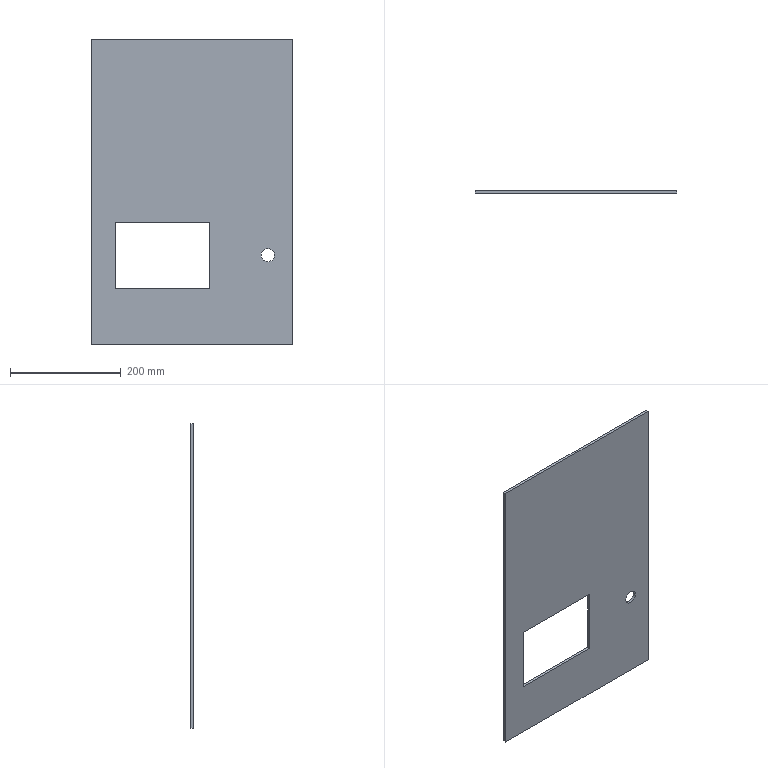Part | NX | 1 solid | 12 faces | box 365 x 5 x 550 mm | volume 899488 mm3 | plane 10 | cylinder 2 | commonest cylinder face diameters 24 x2
STEP:
#1=CARTESIAN_POINT('',(189.68,5.,13.));
#2=VERTEX_POINT('',#1);
#3=CARTESIAN_POINT('',(189.68,5.,-11.));
#4=VERTEX_POINT('',#3);
#5=CARTESIAN_POINT('',(189.68,5.,1.));
#6=DIRECTION('',(0.,-1.,0.));
#7=DIRECTION('',(0.,0.,-1.));
#8=AXIS2_PLACEMENT_3D('',#5,#6,#7);
#9=CIRCLE('',#8,12.);
#10=EDGE_CURVE('',#2,#4,#9,.T.);
#11=ORIENTED_EDGE('',*,*,#10,.F.);
#12=CARTESIAN_POINT('',(189.68,0.,13.));
#13=VERTEX_POINT('',#12);
#14=CARTESIAN_POINT('',(189.68,5.,13.));
#15=DIRECTION('',(0.,1.,0.));
#16=VECTOR('',#15,1.);
#17=LINE('',#14,#16);
#18=EDGE_CURVE('',#13,#2,#17,.T.);
#19=ORIENTED_EDGE('',*,*,#18,.F.);
#20=CARTESIAN_POINT('',(189.68,0.,-11.));
#21=VERTEX_POINT('',#20);
#22=CARTESIAN_POINT('',(189.68,0.,1.));
#23=DIRECTION('',(0.,-1.,0.));
#24=DIRECTION('',(0.,0.,-1.));
#25=AXIS2_PLACEMENT_3D('',#22,#23,#24);
#26=CIRCLE('',#25,12.);
#27=EDGE_CURVE('',#13,#21,#26,.T.);
#28=ORIENTED_EDGE('',*,*,#27,.T.);
#29=CARTESIAN_POINT('',(189.68,5.,-11.));
#30=DIRECTION('',(0.,1.,0.));
#31=VECTOR('',#30,1.);
#32=LINE('',#29,#31);
#33=EDGE_CURVE('',#21,#4,#32,.T.);
#34=ORIENTED_EDGE('',*,*,#33,.T.);
#35=EDGE_LOOP('',(#11,#19,#28,#34));
#36=FACE_OUTER_BOUND('',#35,.T.);
#37=CARTESIAN_POINT('',(189.68,5.,1.));
#38=DIRECTION('',(0.,-1.,0.));
#39=DIRECTION('',(0.,0.,-1.));
#40=AXIS2_PLACEMENT_3D('',#37,#38,#39);
#41=CYLINDRICAL_SURFACE('',#40,12.);
#42=ADVANCED_FACE('',(#36),#41,.F.);
#43=CARTESIAN_POINT('',(189.68,5.,1.));
#44=DIRECTION('',(0.,-1.,0.));
#45=DIRECTION('',(0.,0.,-1.));
#46=AXIS2_PLACEMENT_3D('',#43,#44,#45);
#47=CIRCLE('',#46,12.);
#48=EDGE_CURVE('',#4,#2,#47,.T.);
#49=ORIENTED_EDGE('',*,*,#48,.T.);
#50=ORIENTED_EDGE('',*,*,#10,.T.);
#51=EDGE_LOOP('',(#49,#50));
#52=FACE_BOUND('',#51,.T.);
#53=CARTESIAN_POINT('',(235.,5.,-160.));
#54=VERTEX_POINT('',#53);
#55=CARTESIAN_POINT('',(-130.,5.,-160.));
#56=VERTEX_POINT('',#55);
#57=CARTESIAN_POINT('',(-165.,5.,-160.));
#58=DIRECTION('',(-1.,0.,0.));
#59=VECTOR('',#58,1.);
#60=LINE('',#57,#59);
#61=EDGE_CURVE('',#54,#56,#60,.T.);
#62=ORIENTED_EDGE('',*,*,#61,.T.);
#63=CARTESIAN_POINT('',(-130.,5.,390.));
#64=VERTEX_POINT('',#63);
#65=CARTESIAN_POINT('',(-130.,5.,-160.));
#66=DIRECTION('',(0.,0.,-1.));
#67=VECTOR('',#66,1.);
#68=LINE('',#65,#67);
#69=EDGE_CURVE('',#64,#56,#68,.T.);
#70=ORIENTED_EDGE('',*,*,#69,.F.);
#71=CARTESIAN_POINT('',(235.,5.,390.));
#72=VERTEX_POINT('',#71);
#73=CARTESIAN_POINT('',(-165.,5.,390.));
#74=DIRECTION('',(1.,0.,0.));
#75=VECTOR('',#74,1.);
#76=LINE('',#73,#75);
#77=EDGE_CURVE('',#64,#72,#76,.T.);
#78=ORIENTED_EDGE('',*,*,#77,.T.);
#79=CARTESIAN_POINT('',(235.,5.,-160.));
#80=DIRECTION('',(0.,0.,-1.));
#81=VECTOR('',#80,1.);
#82=LINE('',#79,#81);
#83=EDGE_CURVE('',#72,#54,#82,.T.);
#84=ORIENTED_EDGE('',*,*,#83,.T.);
#85=EDGE_LOOP('',(#62,#70,#78,#84));
#86=FACE_BOUND('',#85,.T.);
#87=CARTESIAN_POINT('',(85.,5.,60.));
#88=VERTEX_POINT('',#87);
#89=CARTESIAN_POINT('',(85.,5.,-60.));
#90=VERTEX_POINT('',#89);
#91=CARTESIAN_POINT('',(85.,5.,-60.));
#92=DIRECTION('',(0.,0.,-1.));
#93=VECTOR('',#92,1.);
#94=LINE('',#91,#93);
#95=EDGE_CURVE('',#88,#90,#94,.T.);
#96=ORIENTED_EDGE('',*,*,#95,.F.);
#97=CARTESIAN_POINT('',(-85.,5.,60.));
#98=VERTEX_POINT('',#97);
#99=CARTESIAN_POINT('',(-85.,5.,60.));
#100=DIRECTION('',(1.,0.,0.));
#101=VECTOR('',#100,1.);
#102=LINE('',#99,#101);
#103=EDGE_CURVE('',#98,#88,#102,.T.);
#104=ORIENTED_EDGE('',*,*,#103,.F.);
#105=CARTESIAN_POINT('',(-85.,5.,-60.));
#106=VERTEX_POINT('',#105);
#107=CARTESIAN_POINT('',(-85.,5.,-60.));
#108=DIRECTION('',(0.,0.,1.));
#109=VECTOR('',#108,1.);
#110=LINE('',#107,#109);
#111=EDGE_CURVE('',#106,#98,#110,.T.);
#112=ORIENTED_EDGE('',*,*,#111,.F.);
#113=CARTESIAN_POINT('',(-85.,5.,-60.));
#114=DIRECTION('',(-1.,0.,0.));
#115=VECTOR('',#114,1.);
#116=LINE('',#113,#115);
#117=EDGE_CURVE('',#90,#106,#116,.T.);
#118=ORIENTED_EDGE('',*,*,#117,.F.);
#119=EDGE_LOOP('',(#96,#104,#112,#118));
#120=FACE_BOUND('',#119,.T.);
#121=CARTESIAN_POINT('',(235.,5.,-160.));
#122=DIRECTION('',(0.,-1.,0.));
#123=DIRECTION('',(0.,0.,-1.));
#124=AXIS2_PLACEMENT_3D('',#121,#122,#123);
#125=PLANE('',#124);
#126=ADVANCED_FACE('',(#52,#86,#120),#125,.F.);
#127=CARTESIAN_POINT('',(189.68,0.,1.));
#128=DIRECTION('',(0.,-1.,0.));
#129=DIRECTION('',(0.,0.,-1.));
#130=AXIS2_PLACEMENT_3D('',#127,#128,#129);
#131=CIRCLE('',#130,12.);
#132=EDGE_CURVE('',#21,#13,#131,.T.);
#133=ORIENTED_EDGE('',*,*,#132,.F.);
#134=ORIENTED_EDGE('',*,*,#27,.F.);
#135=EDGE_LOOP('',(#133,#134));
#136=FACE_BOUND('',#135,.T.);
#137=CARTESIAN_POINT('',(-130.,0.,-160.));
#138=VERTEX_POINT('',#137);
#139=CARTESIAN_POINT('',(-130.,0.,390.));
#140=VERTEX_POINT('',#139);
#141=CARTESIAN_POINT('',(-130.,0.,-160.));
#142=DIRECTION('',(0.,0.,1.));
#143=VECTOR('',#142,1.);
#144=LINE('',#141,#143);
#145=EDGE_CURVE('',#138,#140,#144,.T.);
#146=ORIENTED_EDGE('',*,*,#145,.F.);
#147=CARTESIAN_POINT('',(235.,0.,-160.));
#148=VERTEX_POINT('',#147);
#149=CARTESIAN_POINT('',(-165.,0.,-160.));
#150=DIRECTION('',(-1.,0.,0.));
#151=VECTOR('',#150,1.);
#152=LINE('',#149,#151);
#153=EDGE_CURVE('',#148,#138,#152,.T.);
#154=ORIENTED_EDGE('',*,*,#153,.F.);
#155=CARTESIAN_POINT('',(235.,0.,390.));
#156=VERTEX_POINT('',#155);
#157=CARTESIAN_POINT('',(235.,0.,-160.));
#158=DIRECTION('',(0.,0.,-1.));
#159=VECTOR('',#158,1.);
#160=LINE('',#157,#159);
#161=EDGE_CURVE('',#156,#148,#160,.T.);
#162=ORIENTED_EDGE('',*,*,#161,.F.);
#163=CARTESIAN_POINT('',(-165.,0.,390.));
#164=DIRECTION('',(1.,0.,0.));
#165=VECTOR('',#164,1.);
#166=LINE('',#163,#165);
#167=EDGE_CURVE('',#140,#156,#166,.T.);
#168=ORIENTED_EDGE('',*,*,#167,.F.);
#169=EDGE_LOOP('',(#146,#154,#162,#168));
#170=FACE_BOUND('',#169,.T.);
#171=CARTESIAN_POINT('',(-85.,0.,60.));
#172=VERTEX_POINT('',#171);
#173=CARTESIAN_POINT('',(85.,0.,60.));
#174=VERTEX_POINT('',#173);
#175=CARTESIAN_POINT('',(-85.,0.,60.));
#176=DIRECTION('',(1.,0.,0.));
#177=VECTOR('',#176,1.);
#178=LINE('',#175,#177);
#179=EDGE_CURVE('',#172,#174,#178,.T.);
#180=ORIENTED_EDGE('',*,*,#179,.T.);
#181=CARTESIAN_POINT('',(85.,0.,-60.));
#182=VERTEX_POINT('',#181);
#183=CARTESIAN_POINT('',(85.,0.,-60.));
#184=DIRECTION('',(0.,0.,-1.));
#185=VECTOR('',#184,1.);
#186=LINE('',#183,#185);
#187=EDGE_CURVE('',#174,#182,#186,.T.);
#188=ORIENTED_EDGE('',*,*,#187,.T.);
#189=CARTESIAN_POINT('',(-85.,0.,-60.));
#190=VERTEX_POINT('',#189);
#191=CARTESIAN_POINT('',(-85.,0.,-60.));
#192=DIRECTION('',(-1.,0.,0.));
#193=VECTOR('',#192,1.);
#194=LINE('',#191,#193);
#195=EDGE_CURVE('',#182,#190,#194,.T.);
#196=ORIENTED_EDGE('',*,*,#195,.T.);
#197=CARTESIAN_POINT('',(-85.,0.,-60.));
#198=DIRECTION('',(0.,0.,1.));
#199=VECTOR('',#198,1.);
#200=LINE('',#197,#199);
#201=EDGE_CURVE('',#190,#172,#200,.T.);
#202=ORIENTED_EDGE('',*,*,#201,.T.);
#203=EDGE_LOOP('',(#180,#188,#196,#202));
#204=FACE_BOUND('',#203,.T.);
#205=CARTESIAN_POINT('',(235.,0.,-160.));
#206=DIRECTION('',(0.,-1.,0.));
#207=DIRECTION('',(0.,0.,-1.));
#208=AXIS2_PLACEMENT_3D('',#205,#206,#207);
#209=PLANE('',#208);
#210=ADVANCED_FACE('',(#136,#170,#204),#209,.T.);
#211=ORIENTED_EDGE('',*,*,#153,.T.);
#212=CARTESIAN_POINT('',(-130.,-5.,-160.));
#213=DIRECTION('',(0.,1.,0.));
#214=VECTOR('',#213,1.);
#215=LINE('',#212,#214);
#216=EDGE_CURVE('',#138,#56,#215,.T.);
#217=ORIENTED_EDGE('',*,*,#216,.T.);
#218=ORIENTED_EDGE('',*,*,#61,.F.);
#219=CARTESIAN_POINT('',(235.,5.,-160.));
#220=DIRECTION('',(0.,-1.,0.));
#221=VECTOR('',#220,1.);
#222=LINE('',#219,#221);
#223=EDGE_CURVE('',#54,#148,#222,.T.);
#224=ORIENTED_EDGE('',*,*,#223,.T.);
#225=EDGE_LOOP('',(#211,#217,#218,#224));
#226=FACE_OUTER_BOUND('',#225,.T.);
#227=CARTESIAN_POINT('',(-165.,5.,-160.));
#228=DIRECTION('',(0.,0.,1.));
#229=DIRECTION('',(1.,0.,0.));
#230=AXIS2_PLACEMENT_3D('',#227,#228,#229);
#231=PLANE('',#230);
#232=ADVANCED_FACE('',(#226),#231,.F.);
#233=ORIENTED_EDGE('',*,*,#77,.F.);
#234=CARTESIAN_POINT('',(-130.,5.,390.));
#235=DIRECTION('',(0.,-1.,0.));
#236=VECTOR('',#235,1.);
#237=LINE('',#234,#236);
#238=EDGE_CURVE('',#64,#140,#237,.T.);
#239=ORIENTED_EDGE('',*,*,#238,.T.);
#240=ORIENTED_EDGE('',*,*,#167,.T.);
#241=CARTESIAN_POINT('',(235.,5.,390.));
#242=DIRECTION('',(0.,-1.,0.));
#243=VECTOR('',#242,1.);
#244=LINE('',#241,#243);
#245=EDGE_CURVE('',#72,#156,#244,.T.);
#246=ORIENTED_EDGE('',*,*,#245,.F.);
#247=EDGE_LOOP('',(#233,#239,#240,#246));
#248=FACE_OUTER_BOUND('',#247,.T.);
#249=CARTESIAN_POINT('',(-165.,5.,390.));
#250=DIRECTION('',(0.,0.,-1.));
#251=DIRECTION('',(-1.,0.,0.));
#252=AXIS2_PLACEMENT_3D('',#249,#250,#251);
#253=PLANE('',#252);
#254=ADVANCED_FACE('',(#248),#253,.F.);
#255=ORIENTED_EDGE('',*,*,#161,.T.);
#256=ORIENTED_EDGE('',*,*,#223,.F.);
#257=ORIENTED_EDGE('',*,*,#83,.F.);
#258=ORIENTED_EDGE('',*,*,#245,.T.);
#259=EDGE_LOOP('',(#255,#256,#257,#258));
#260=FACE_OUTER_BOUND('',#259,.T.);
#261=CARTESIAN_POINT('',(235.,5.,-160.));
#262=DIRECTION('',(-1.,0.,0.));
#263=DIRECTION('',(0.,0.,1.));
#264=AXIS2_PLACEMENT_3D('',#261,#262,#263);
#265=PLANE('',#264);
#266=ADVANCED_FACE('',(#260),#265,.F.);
#267=ORIENTED_EDGE('',*,*,#187,.F.);
#268=CARTESIAN_POINT('',(85.,5.,60.));
#269=DIRECTION('',(0.,-1.,0.));
#270=VECTOR('',#269,1.);
#271=LINE('',#268,#270);
#272=EDGE_CURVE('',#88,#174,#271,.T.);
#273=ORIENTED_EDGE('',*,*,#272,.F.);
#274=ORIENTED_EDGE('',*,*,#95,.T.);
#275=CARTESIAN_POINT('',(85.,5.,-60.));
#276=DIRECTION('',(0.,-1.,0.));
#277=VECTOR('',#276,1.);
#278=LINE('',#275,#277);
#279=EDGE_CURVE('',#90,#182,#278,.T.);
#280=ORIENTED_EDGE('',*,*,#279,.T.);
#281=EDGE_LOOP('',(#267,#273,#274,#280));
#282=FACE_OUTER_BOUND('',#281,.T.);
#283=CARTESIAN_POINT('',(85.,5.,-60.));
#284=DIRECTION('',(-1.,0.,0.));
#285=DIRECTION('',(0.,0.,1.));
#286=AXIS2_PLACEMENT_3D('',#283,#284,#285);
#287=PLANE('',#286);
#288=ADVANCED_FACE('',(#282),#287,.T.);
#289=ORIENTED_EDGE('',*,*,#195,.F.);
#290=ORIENTED_EDGE('',*,*,#279,.F.);
#291=ORIENTED_EDGE('',*,*,#117,.T.);
#292=CARTESIAN_POINT('',(-85.,5.,-60.));
#293=DIRECTION('',(0.,-1.,0.));
#294=VECTOR('',#293,1.);
#295=LINE('',#292,#294);
#296=EDGE_CURVE('',#106,#190,#295,.T.);
#297=ORIENTED_EDGE('',*,*,#296,.T.);
#298=EDGE_LOOP('',(#289,#290,#291,#297));
#299=FACE_OUTER_BOUND('',#298,.T.);
#300=CARTESIAN_POINT('',(-85.,5.,-60.));
#301=DIRECTION('',(0.,0.,1.));
#302=DIRECTION('',(1.,0.,0.));
#303=AXIS2_PLACEMENT_3D('',#300,#301,#302);
#304=PLANE('',#303);
#305=ADVANCED_FACE('',(#299),#304,.T.);
#306=ORIENTED_EDGE('',*,*,#201,.F.);
#307=ORIENTED_EDGE('',*,*,#296,.F.);
#308=ORIENTED_EDGE('',*,*,#111,.T.);
#309=CARTESIAN_POINT('',(-85.,5.,60.));
#310=DIRECTION('',(0.,-1.,0.));
#311=VECTOR('',#310,1.);
#312=LINE('',#309,#311);
#313=EDGE_CURVE('',#98,#172,#312,.T.);
#314=ORIENTED_EDGE('',*,*,#313,.T.);
#315=EDGE_LOOP('',(#306,#307,#308,#314));
#316=FACE_OUTER_BOUND('',#315,.T.);
#317=CARTESIAN_POINT('',(-85.,5.,-60.));
#318=DIRECTION('',(1.,0.,0.));
#319=DIRECTION('',(0.,0.,-1.));
#320=AXIS2_PLACEMENT_3D('',#317,#318,#319);
#321=PLANE('',#320);
#322=ADVANCED_FACE('',(#316),#321,.T.);
#323=ORIENTED_EDGE('',*,*,#179,.F.);
#324=ORIENTED_EDGE('',*,*,#313,.F.);
#325=ORIENTED_EDGE('',*,*,#103,.T.);
#326=ORIENTED_EDGE('',*,*,#272,.T.);
#327=EDGE_LOOP('',(#323,#324,#325,#326));
#328=FACE_OUTER_BOUND('',#327,.T.);
#329=CARTESIAN_POINT('',(-85.,5.,60.));
#330=DIRECTION('',(0.,0.,-1.));
#331=DIRECTION('',(-1.,0.,0.));
#332=AXIS2_PLACEMENT_3D('',#329,#330,#331);
#333=PLANE('',#332);
#334=ADVANCED_FACE('',(#328),#333,.T.);
#335=ORIENTED_EDGE('',*,*,#145,.T.);
#336=ORIENTED_EDGE('',*,*,#238,.F.);
#337=ORIENTED_EDGE('',*,*,#69,.T.);
#338=ORIENTED_EDGE('',*,*,#216,.F.);
#339=EDGE_LOOP('',(#335,#336,#337,#338));
#340=FACE_OUTER_BOUND('',#339,.T.);
#341=CARTESIAN_POINT('',(-130.,-5.,-160.));
#342=DIRECTION('',(1.,0.,0.));
#343=DIRECTION('',(0.,0.,-1.));
#344=AXIS2_PLACEMENT_3D('',#341,#342,#343);
#345=PLANE('',#344);
#346=ADVANCED_FACE('',(#340),#345,.F.);
#347=ORIENTED_EDGE('',*,*,#18,.T.);
#348=ORIENTED_EDGE('',*,*,#48,.F.);
#349=ORIENTED_EDGE('',*,*,#33,.F.);
#350=ORIENTED_EDGE('',*,*,#132,.T.);
#351=EDGE_LOOP('',(#347,#348,#349,#350));
#352=FACE_OUTER_BOUND('',#351,.T.);
#353=CARTESIAN_POINT('',(189.68,5.,1.));
#354=DIRECTION('',(0.,-1.,0.));
#355=DIRECTION('',(0.,0.,-1.));
#356=AXIS2_PLACEMENT_3D('',#353,#354,#355);
#357=CYLINDRICAL_SURFACE('',#356,12.);
#358=ADVANCED_FACE('',(#352),#357,.F.);
#359=CLOSED_SHELL('',(#42,#126,#210,#232,#254,#266,#288,#305,#322,#334,#346,#358));
#360=MANIFOLD_SOLID_BREP('',#359);
#361=(LENGTH_UNIT()NAMED_UNIT(*)SI_UNIT(.MILLI.,.METRE.));
#362=UNCERTAINTY_MEASURE_WITH_UNIT(LENGTH_MEASURE(0.00002),#361,'','');
#363=(NAMED_UNIT(*)PLANE_ANGLE_UNIT()SI_UNIT($,.RADIAN.));
#364=PLANE_ANGLE_MEASURE_WITH_UNIT(PLANE_ANGLE_MEASURE(0.01745),#363);
#365=DIMENSIONAL_EXPONENTS(0.,0.,0.,0.,0.,0.,0.);
#366=(CONVERSION_BASED_UNIT('DEGREE',#364)NAMED_UNIT(#365)PLANE_ANGLE_UNIT());
#367=(NAMED_UNIT(*)SI_UNIT($,.STERADIAN.)SOLID_ANGLE_UNIT());
#368=(GEOMETRIC_REPRESENTATION_CONTEXT(3)GLOBAL_UNCERTAINTY_ASSIGNED_CONTEXT((#362))GLOBAL_UNIT_ASSIGNED_CONTEXT((#361,#366,#367))REPRESENTATION_CONTEXT('',''));
#369=ADVANCED_BREP_SHAPE_REPRESENTATION('',(#360),#368);